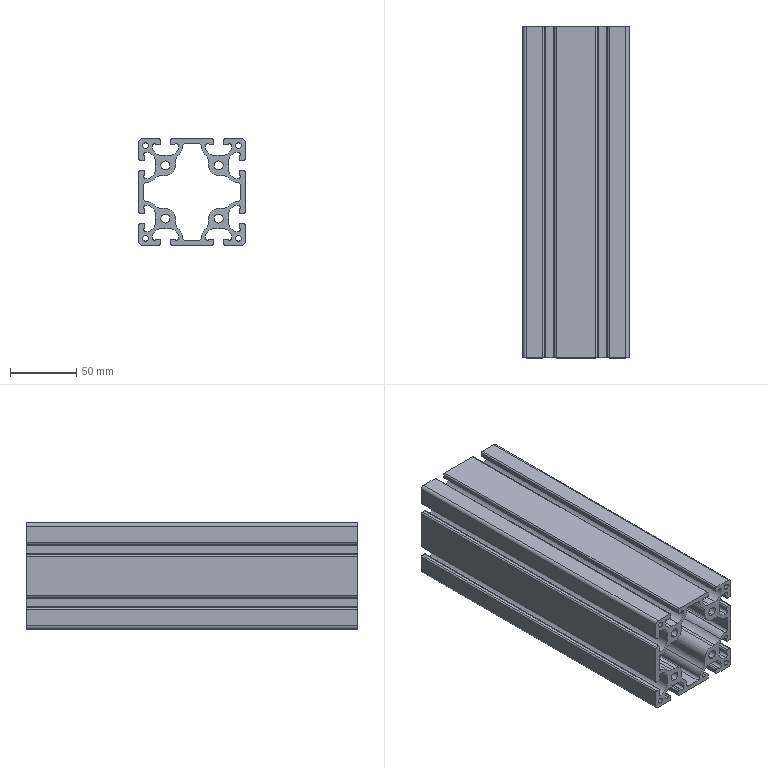Part | STEP file | 00175958_EZT_PROFILSAEULE_HMBS-80.80-250-.1 | 1 solid | 194 faces | box 80 x 250 x 80 mm | volume 517689 mm3 | cylinder 120 | plane 74 | commonest cylinder face diameters 2 x32 14.3 x26 3.5 x20 14 x10 4 x8 4.2 x8